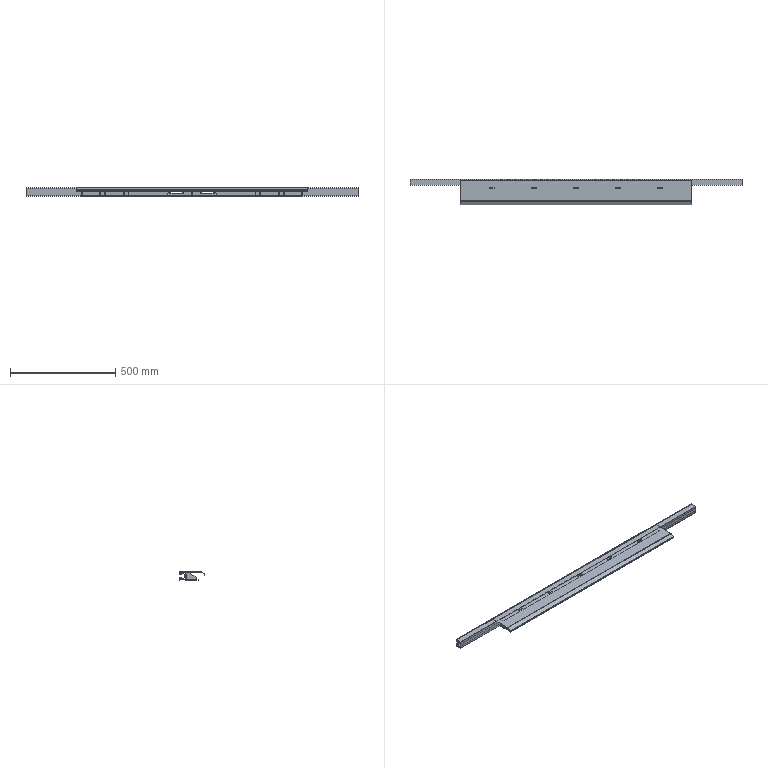Part | 11 solids | 301 faces | box 1580 x 122.821 x 40 mm | volume 1026552 mm3 | plane 181 | cylinder 120 | commonest cylinder face diameters 6 x74 2 x18 11 x12 10 x6 12 x4 3 x2